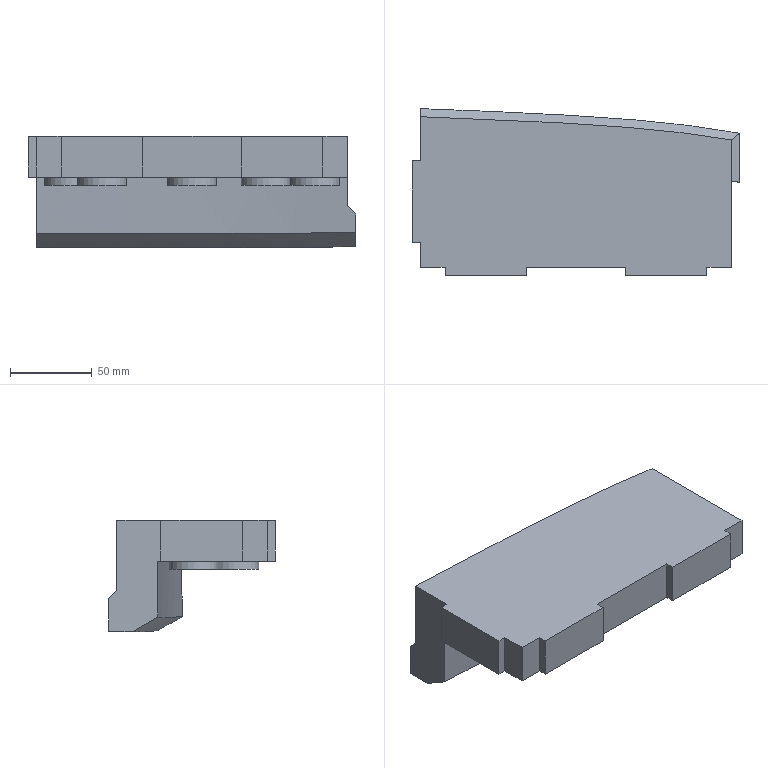Part | NX | features solid 2 | 1 solid | 35 faces | box 199.995 x 101.881 x 68.039 mm | volume 664832 mm3 | plane 24 | spline 6 | cylinder 5 | commonest cylinder face diameters 30 x5